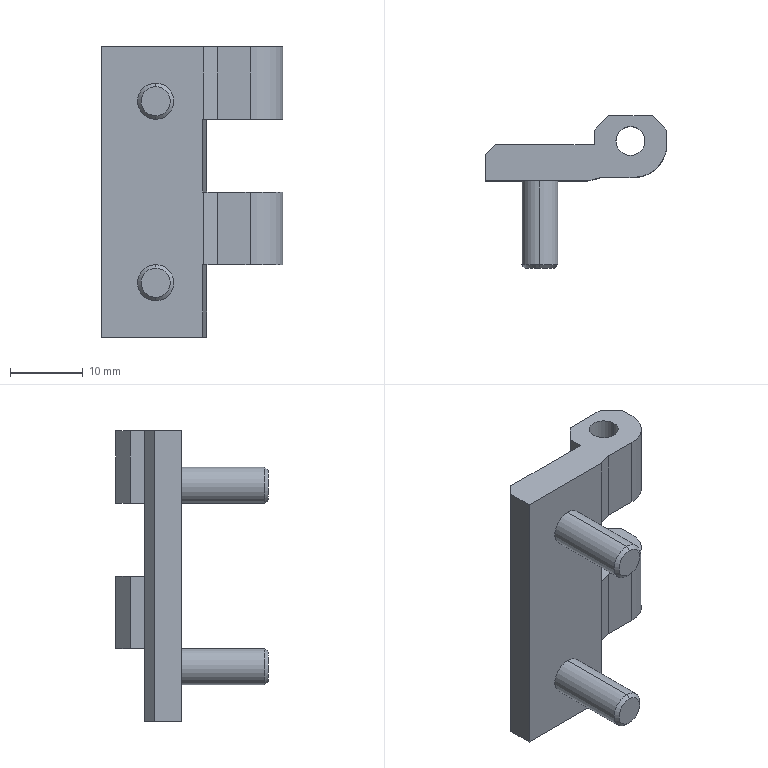Part | SolidWorks | features BaseBody 1 | 1 solid | 41 faces | box 25 x 21 x 40 mm | volume 4636 mm3 | plane 27 | cylinder 10 | cone 4 | commonest cylinder face diameters 4 x4 5 x4 9 x2
STEP:
#1=CARTESIAN_POINT('',(2.,5.5,20.));
#2=VERTEX_POINT('',#1);
#3=CARTESIAN_POINT('',(-2.,5.5,20.));
#4=VERTEX_POINT('',#3);
#5=CARTESIAN_POINT('',(0.,5.5,20.));
#6=DIRECTION('',(0.,0.,-1.));
#7=DIRECTION('',(-1.,0.,0.));
#8=AXIS2_PLACEMENT_3D('',#5,#6,#7);
#9=CIRCLE('',#8,2.);
#10=EDGE_CURVE('',#2,#4,#9,.T.);
#11=ORIENTED_EDGE('',*,*,#10,.F.);
#12=CARTESIAN_POINT('',(2.,5.5,10.));
#13=VERTEX_POINT('',#12);
#14=CARTESIAN_POINT('',(2.,5.5,20.));
#15=DIRECTION('',(0.,0.,-1.));
#16=VECTOR('',#15,1000.);
#17=LINE('',#14,#16);
#18=EDGE_CURVE('',#2,#13,#17,.T.);
#19=ORIENTED_EDGE('',*,*,#18,.T.);
#20=CARTESIAN_POINT('',(-2.,5.5,10.));
#21=VERTEX_POINT('',#20);
#22=CARTESIAN_POINT('',(0.,5.5,10.));
#23=DIRECTION('',(0.,0.,1.));
#24=DIRECTION('',(-1.,0.,0.));
#25=AXIS2_PLACEMENT_3D('',#22,#23,#24);
#26=CIRCLE('',#25,2.);
#27=EDGE_CURVE('',#21,#13,#26,.T.);
#28=ORIENTED_EDGE('',*,*,#27,.F.);
#29=CARTESIAN_POINT('',(-2.,5.5,20.));
#30=DIRECTION('',(0.,0.,-1.));
#31=VECTOR('',#30,1000.);
#32=LINE('',#29,#31);
#33=EDGE_CURVE('',#4,#21,#32,.T.);
#34=ORIENTED_EDGE('',*,*,#33,.F.);
#35=EDGE_LOOP('',(#11,#19,#28,#34));
#36=FACE_OUTER_BOUND('',#35,.T.);
#37=CARTESIAN_POINT('',(0.,5.5,20.));
#38=DIRECTION('',(0.,0.,-1.));
#39=DIRECTION('',(-1.,0.,0.));
#40=AXIS2_PLACEMENT_3D('',#37,#38,#39);
#41=CYLINDRICAL_SURFACE('',#40,2.);
#42=ADVANCED_FACE('',(#36),#41,.F.);
#43=CARTESIAN_POINT('',(-12.5,0.,10.));
#44=VERTEX_POINT('',#43);
#45=CARTESIAN_POINT('',(-12.5,0.,15.));
#46=VERTEX_POINT('',#45);
#47=CARTESIAN_POINT('',(-12.5,0.,12.5));
#48=DIRECTION('',(0.,-1.,0.));
#49=DIRECTION('',(0.,0.,-1.));
#50=AXIS2_PLACEMENT_3D('',#47,#48,#49);
#51=CIRCLE('',#50,2.5);
#52=EDGE_CURVE('',#44,#46,#51,.T.);
#53=ORIENTED_EDGE('',*,*,#52,.T.);
#54=CARTESIAN_POINT('',(-12.5,-11.509,15.));
#55=VERTEX_POINT('',#54);
#56=CARTESIAN_POINT('',(-12.5,-12.,15.));
#57=DIRECTION('',(0.,-1.,0.));
#58=VECTOR('',#57,1000.);
#59=LINE('',#56,#58);
#60=EDGE_CURVE('',#46,#55,#59,.T.);
#61=ORIENTED_EDGE('',*,*,#60,.T.);
#62=CARTESIAN_POINT('',(-12.5,-11.509,10.));
#63=VERTEX_POINT('',#62);
#64=CARTESIAN_POINT('',(-12.5,-11.509,12.5));
#65=DIRECTION('',(0.,1.,0.));
#66=DIRECTION('',(0.,0.,-1.));
#67=AXIS2_PLACEMENT_3D('',#64,#65,#66);
#68=CIRCLE('',#67,2.5);
#69=EDGE_CURVE('',#55,#63,#68,.T.);
#70=ORIENTED_EDGE('',*,*,#69,.T.);
#71=CARTESIAN_POINT('',(-12.5,-12.,10.));
#72=DIRECTION('',(0.,-1.,0.));
#73=VECTOR('',#72,1000.);
#74=LINE('',#71,#73);
#75=EDGE_CURVE('',#44,#63,#74,.T.);
#76=ORIENTED_EDGE('',*,*,#75,.F.);
#77=EDGE_LOOP('',(#53,#61,#70,#76));
#78=FACE_OUTER_BOUND('',#77,.T.);
#79=CARTESIAN_POINT('',(-12.5,-12.,12.5));
#80=DIRECTION('',(0.,-1.,0.));
#81=DIRECTION('',(0.,0.,-1.));
#82=AXIS2_PLACEMENT_3D('',#79,#80,#81);
#83=CYLINDRICAL_SURFACE('',#82,2.5);
#84=ADVANCED_FACE('',(#78),#83,.T.);
#85=CARTESIAN_POINT('',(-12.5,0.,-15.));
#86=VERTEX_POINT('',#85);
#87=CARTESIAN_POINT('',(-12.5,0.,-10.));
#88=VERTEX_POINT('',#87);
#89=CARTESIAN_POINT('',(-12.5,0.,-12.5));
#90=DIRECTION('',(0.,-1.,0.));
#91=DIRECTION('',(0.,0.,-1.));
#92=AXIS2_PLACEMENT_3D('',#89,#90,#91);
#93=CIRCLE('',#92,2.5);
#94=EDGE_CURVE('',#86,#88,#93,.T.);
#95=ORIENTED_EDGE('',*,*,#94,.T.);
#96=CARTESIAN_POINT('',(-12.5,-11.509,-10.));
#97=VERTEX_POINT('',#96);
#98=CARTESIAN_POINT('',(-12.5,-12.,-10.));
#99=DIRECTION('',(0.,-1.,0.));
#100=VECTOR('',#99,1000.);
#101=LINE('',#98,#100);
#102=EDGE_CURVE('',#88,#97,#101,.T.);
#103=ORIENTED_EDGE('',*,*,#102,.T.);
#104=CARTESIAN_POINT('',(-12.5,-11.509,-15.));
#105=VERTEX_POINT('',#104);
#106=CARTESIAN_POINT('',(-12.5,-11.509,-12.5));
#107=DIRECTION('',(0.,1.,0.));
#108=DIRECTION('',(0.,0.,-1.));
#109=AXIS2_PLACEMENT_3D('',#106,#107,#108);
#110=CIRCLE('',#109,2.5);
#111=EDGE_CURVE('',#97,#105,#110,.T.);
#112=ORIENTED_EDGE('',*,*,#111,.T.);
#113=CARTESIAN_POINT('',(-12.5,-12.,-15.));
#114=DIRECTION('',(0.,-1.,0.));
#115=VECTOR('',#114,1000.);
#116=LINE('',#113,#115);
#117=EDGE_CURVE('',#86,#105,#116,.T.);
#118=ORIENTED_EDGE('',*,*,#117,.F.);
#119=EDGE_LOOP('',(#95,#103,#112,#118));
#120=FACE_OUTER_BOUND('',#119,.T.);
#121=CARTESIAN_POINT('',(-12.5,-12.,-12.5));
#122=DIRECTION('',(0.,-1.,0.));
#123=DIRECTION('',(0.,0.,-1.));
#124=AXIS2_PLACEMENT_3D('',#121,#122,#123);
#125=CYLINDRICAL_SURFACE('',#124,2.5);
#126=ADVANCED_FACE('',(#120),#125,.T.);
#127=CARTESIAN_POINT('',(2.,5.5,-10.));
#128=VERTEX_POINT('',#127);
#129=CARTESIAN_POINT('',(-2.,5.5,-10.));
#130=VERTEX_POINT('',#129);
#131=CARTESIAN_POINT('',(0.,5.5,-10.));
#132=DIRECTION('',(0.,0.,-1.));
#133=DIRECTION('',(1.,0.,0.));
#134=AXIS2_PLACEMENT_3D('',#131,#132,#133);
#135=CIRCLE('',#134,2.);
#136=EDGE_CURVE('',#128,#130,#135,.T.);
#137=ORIENTED_EDGE('',*,*,#136,.T.);
#138=CARTESIAN_POINT('',(-2.,5.5,0.));
#139=VERTEX_POINT('',#138);
#140=CARTESIAN_POINT('',(-2.,5.5,-10.));
#141=DIRECTION('',(0.,0.,1.));
#142=VECTOR('',#141,1000.);
#143=LINE('',#140,#142);
#144=EDGE_CURVE('',#130,#139,#143,.T.);
#145=ORIENTED_EDGE('',*,*,#144,.T.);
#146=CARTESIAN_POINT('',(2.,5.5,0.));
#147=VERTEX_POINT('',#146);
#148=CARTESIAN_POINT('',(0.,5.5,0.));
#149=DIRECTION('',(0.,0.,-1.));
#150=DIRECTION('',(1.,0.,0.));
#151=AXIS2_PLACEMENT_3D('',#148,#149,#150);
#152=CIRCLE('',#151,2.);
#153=EDGE_CURVE('',#147,#139,#152,.T.);
#154=ORIENTED_EDGE('',*,*,#153,.F.);
#155=CARTESIAN_POINT('',(2.,5.5,-10.));
#156=DIRECTION('',(0.,0.,1.));
#157=VECTOR('',#156,1000.);
#158=LINE('',#155,#157);
#159=EDGE_CURVE('',#128,#147,#158,.T.);
#160=ORIENTED_EDGE('',*,*,#159,.F.);
#161=EDGE_LOOP('',(#137,#145,#154,#160));
#162=FACE_OUTER_BOUND('',#161,.T.);
#163=CARTESIAN_POINT('',(0.,5.5,-10.));
#164=DIRECTION('',(0.,0.,1.));
#165=DIRECTION('',(1.,0.,0.));
#166=AXIS2_PLACEMENT_3D('',#163,#164,#165);
#167=CYLINDRICAL_SURFACE('',#166,2.);
#168=ADVANCED_FACE('',(#162),#167,.F.);
#169=CARTESIAN_POINT('',(-12.5,-12.,14.509));
#170=VERTEX_POINT('',#169);
#171=CARTESIAN_POINT('',(-12.5,-12.,10.491));
#172=VERTEX_POINT('',#171);
#173=CARTESIAN_POINT('',(-12.5,-12.,12.5));
#174=DIRECTION('',(0.,1.,0.));
#175=DIRECTION('',(0.,0.,1.));
#176=AXIS2_PLACEMENT_3D('',#173,#174,#175);
#177=CIRCLE('',#176,2.009);
#178=EDGE_CURVE('',#170,#172,#177,.T.);
#179=ORIENTED_EDGE('',*,*,#178,.T.);
#180=CARTESIAN_POINT('',(-12.5,-11.51,10.));
#181=DIRECTION('',(0.,0.7071,-0.7071));
#182=VECTOR('',#181,1000.);
#183=LINE('',#180,#182);
#184=EDGE_CURVE('',#172,#63,#183,.T.);
#185=ORIENTED_EDGE('',*,*,#184,.T.);
#186=ORIENTED_EDGE('',*,*,#69,.F.);
#187=CARTESIAN_POINT('',(-12.5,-11.51,15.));
#188=DIRECTION('',(0.,0.7071,0.7071));
#189=VECTOR('',#188,1000.);
#190=LINE('',#187,#189);
#191=EDGE_CURVE('',#170,#55,#190,.T.);
#192=ORIENTED_EDGE('',*,*,#191,.F.);
#193=EDGE_LOOP('',(#179,#185,#186,#192));
#194=FACE_OUTER_BOUND('',#193,.T.);
#195=CARTESIAN_POINT('',(-12.5,-11.51,12.5));
#196=DIRECTION('',(0.,1.,0.));
#197=DIRECTION('',(0.,0.,1.));
#198=AXIS2_PLACEMENT_3D('',#195,#196,#197);
#199=CONICAL_SURFACE('',#198,2.5,0.7854);
#200=ADVANCED_FACE('',(#194),#199,.T.);
#201=CARTESIAN_POINT('',(-12.5,-12.,-10.49));
#202=VERTEX_POINT('',#201);
#203=CARTESIAN_POINT('',(-12.5,-12.,-14.51));
#204=VERTEX_POINT('',#203);
#205=CARTESIAN_POINT('',(-12.5,-12.,-12.5));
#206=DIRECTION('',(0.,1.,0.));
#207=DIRECTION('',(0.,0.,1.));
#208=AXIS2_PLACEMENT_3D('',#205,#206,#207);
#209=CIRCLE('',#208,2.01);
#210=EDGE_CURVE('',#202,#204,#209,.T.);
#211=ORIENTED_EDGE('',*,*,#210,.T.);
#212=CARTESIAN_POINT('',(-12.5,-11.509,-15.));
#213=DIRECTION('',(0.,0.7071,-0.7071));
#214=VECTOR('',#213,1000.);
#215=LINE('',#212,#214);
#216=EDGE_CURVE('',#204,#105,#215,.T.);
#217=ORIENTED_EDGE('',*,*,#216,.T.);
#218=ORIENTED_EDGE('',*,*,#111,.F.);
#219=CARTESIAN_POINT('',(-12.5,-11.509,-10.));
#220=DIRECTION('',(0.,0.7071,0.7071));
#221=VECTOR('',#220,1000.);
#222=LINE('',#219,#221);
#223=EDGE_CURVE('',#202,#97,#222,.T.);
#224=ORIENTED_EDGE('',*,*,#223,.F.);
#225=EDGE_LOOP('',(#211,#217,#218,#224));
#226=FACE_OUTER_BOUND('',#225,.T.);
#227=CARTESIAN_POINT('',(-12.5,-11.509,-12.5));
#228=DIRECTION('',(0.,1.,0.));
#229=DIRECTION('',(0.,0.,1.));
#230=AXIS2_PLACEMENT_3D('',#227,#228,#229);
#231=CONICAL_SURFACE('',#230,2.5,0.7854);
#232=ADVANCED_FACE('',(#226),#231,.T.);
#233=CARTESIAN_POINT('',(-5.,5.,20.));
#234=VERTEX_POINT('',#233);
#235=CARTESIAN_POINT('',(-18.6,5.,20.));
#236=VERTEX_POINT('',#235);
#237=CARTESIAN_POINT('',(-5.5,5.,20.));
#238=DIRECTION('',(-1.,0.,0.));
#239=VECTOR('',#238,1000.);
#240=LINE('',#237,#239);
#241=EDGE_CURVE('',#234,#236,#240,.T.);
#242=ORIENTED_EDGE('',*,*,#241,.F.);
#243=CARTESIAN_POINT('',(-5.,5.,10.));
#244=VERTEX_POINT('',#243);
#245=CARTESIAN_POINT('',(-5.,5.,20.));
#246=DIRECTION('',(0.,0.,1.));
#247=VECTOR('',#246,1000.);
#248=LINE('',#245,#247);
#249=EDGE_CURVE('',#244,#234,#248,.T.);
#250=ORIENTED_EDGE('',*,*,#249,.F.);
#251=CARTESIAN_POINT('',(-5.5,5.,10.));
#252=VERTEX_POINT('',#251);
#253=CARTESIAN_POINT('',(0.5,5.,10.));
#254=DIRECTION('',(-1.,0.,0.));
#255=VECTOR('',#254,1000.);
#256=LINE('',#253,#255);
#257=EDGE_CURVE('',#244,#252,#256,.T.);
#258=ORIENTED_EDGE('',*,*,#257,.T.);
#259=CARTESIAN_POINT('',(-5.5,5.,0.));
#260=VERTEX_POINT('',#259);
#261=CARTESIAN_POINT('',(-5.5,5.,20.));
#262=DIRECTION('',(0.,0.,1.));
#263=VECTOR('',#262,1000.);
#264=LINE('',#261,#263);
#265=EDGE_CURVE('',#260,#252,#264,.T.);
#266=ORIENTED_EDGE('',*,*,#265,.F.);
#267=CARTESIAN_POINT('',(-5.,5.,0.));
#268=VERTEX_POINT('',#267);
#269=CARTESIAN_POINT('',(0.5,5.,0.));
#270=DIRECTION('',(-1.,0.,0.));
#271=VECTOR('',#270,1000.);
#272=LINE('',#269,#271);
#273=EDGE_CURVE('',#268,#260,#272,.T.);
#274=ORIENTED_EDGE('',*,*,#273,.F.);
#275=CARTESIAN_POINT('',(-5.,5.,-10.));
#276=VERTEX_POINT('',#275);
#277=CARTESIAN_POINT('',(-5.,5.,20.));
#278=DIRECTION('',(0.,0.,1.));
#279=VECTOR('',#278,1000.);
#280=LINE('',#277,#279);
#281=EDGE_CURVE('',#276,#268,#280,.T.);
#282=ORIENTED_EDGE('',*,*,#281,.F.);
#283=CARTESIAN_POINT('',(-5.5,5.,-10.));
#284=VERTEX_POINT('',#283);
#285=CARTESIAN_POINT('',(0.5,5.,-10.));
#286=DIRECTION('',(-1.,0.,0.));
#287=VECTOR('',#286,1000.);
#288=LINE('',#285,#287);
#289=EDGE_CURVE('',#276,#284,#288,.T.);
#290=ORIENTED_EDGE('',*,*,#289,.T.);
#291=CARTESIAN_POINT('',(-5.5,5.,-20.));
#292=VERTEX_POINT('',#291);
#293=CARTESIAN_POINT('',(-5.5,5.,20.));
#294=DIRECTION('',(0.,0.,1.));
#295=VECTOR('',#294,1000.);
#296=LINE('',#293,#295);
#297=EDGE_CURVE('',#292,#284,#296,.T.);
#298=ORIENTED_EDGE('',*,*,#297,.F.);
#299=CARTESIAN_POINT('',(-18.6,5.,-20.));
#300=VERTEX_POINT('',#299);
#301=CARTESIAN_POINT('',(-5.5,5.,-20.));
#302=DIRECTION('',(1.,0.,0.));
#303=VECTOR('',#302,1000.);
#304=LINE('',#301,#303);
#305=EDGE_CURVE('',#300,#292,#304,.T.);
#306=ORIENTED_EDGE('',*,*,#305,.F.);
#307=CARTESIAN_POINT('',(-18.6,5.,20.));
#308=DIRECTION('',(0.,0.,-1.));
#309=VECTOR('',#308,1000.);
#310=LINE('',#307,#309);
#311=EDGE_CURVE('',#236,#300,#310,.T.);
#312=ORIENTED_EDGE('',*,*,#311,.F.);
#313=EDGE_LOOP('',(#242,#250,#258,#266,#274,#282,#290,#298,#306,#312));
#314=FACE_OUTER_BOUND('',#313,.T.);
#315=CARTESIAN_POINT('',(-5.5,5.,20.));
#316=DIRECTION('',(0.,-1.,0.));
#317=DIRECTION('',(0.,0.,-1.));
#318=AXIS2_PLACEMENT_3D('',#315,#316,#317);
#319=PLANE('',#318);
#320=ADVANCED_FACE('',(#314),#319,.F.);
#321=CARTESIAN_POINT('',(-20.,3.6,20.));
#322=VERTEX_POINT('',#321);
#323=CARTESIAN_POINT('',(-20.,3.6,-20.));
#324=VERTEX_POINT('',#323);
#325=CARTESIAN_POINT('',(-20.,3.6,20.));
#326=DIRECTION('',(0.,0.,-1.));
#327=VECTOR('',#326,1000.);
#328=LINE('',#325,#327);
#329=EDGE_CURVE('',#322,#324,#328,.T.);
#330=ORIENTED_EDGE('',*,*,#329,.F.);
#331=CARTESIAN_POINT('',(-18.6,5.,20.));
#332=DIRECTION('',(-0.7071,-0.7071,0.));
#333=VECTOR('',#332,1000.);
#334=LINE('',#331,#333);
#335=EDGE_CURVE('',#236,#322,#334,.T.);
#336=ORIENTED_EDGE('',*,*,#335,.F.);
#337=ORIENTED_EDGE('',*,*,#311,.T.);
#338=CARTESIAN_POINT('',(-18.6,5.,-20.));
#339=DIRECTION('',(0.7071,0.7071,0.));
#340=VECTOR('',#339,1000.);
#341=LINE('',#338,#340);
#342=EDGE_CURVE('',#324,#300,#341,.T.);
#343=ORIENTED_EDGE('',*,*,#342,.F.);
#344=EDGE_LOOP('',(#330,#336,#337,#343));
#345=FACE_OUTER_BOUND('',#344,.T.);
#346=CARTESIAN_POINT('',(-18.6,5.,20.));
#347=DIRECTION('',(0.7071,-0.7071,0.));
#348=DIRECTION('',(0.7071,0.7071,0.));
#349=AXIS2_PLACEMENT_3D('',#346,#347,#348);
#350=PLANE('',#349);
#351=ADVANCED_FACE('',(#345),#350,.F.);
#352=CARTESIAN_POINT('',(0.,5.5,20.));
#353=DIRECTION('',(0.,0.,-1.));
#354=DIRECTION('',(-1.,0.,0.));
#355=AXIS2_PLACEMENT_3D('',#352,#353,#354);
#356=CIRCLE('',#355,2.);
#357=EDGE_CURVE('',#4,#2,#356,.T.);
#358=ORIENTED_EDGE('',*,*,#357,.T.);
#359=ORIENTED_EDGE('',*,*,#10,.T.);
#360=EDGE_LOOP('',(#358,#359));
#361=FACE_BOUND('',#360,.T.);
#362=CARTESIAN_POINT('',(-3.,9.,20.));
#363=VERTEX_POINT('',#362);
#364=CARTESIAN_POINT('',(-5.,7.,20.));
#365=VERTEX_POINT('',#364);
#366=CARTESIAN_POINT('',(-3.,9.,20.));
#367=DIRECTION('',(-0.7071,-0.7071,0.));
#368=VECTOR('',#367,1000.);
#369=LINE('',#366,#368);
#370=EDGE_CURVE('',#363,#365,#369,.T.);
#371=ORIENTED_EDGE('',*,*,#370,.T.);
#372=CARTESIAN_POINT('',(-5.,0.,20.));
#373=DIRECTION('',(0.,-1.,0.));
#374=VECTOR('',#373,1000.);
#375=LINE('',#372,#374);
#376=EDGE_CURVE('',#365,#234,#375,.T.);
#377=ORIENTED_EDGE('',*,*,#376,.T.);
#378=ORIENTED_EDGE('',*,*,#241,.T.);
#379=ORIENTED_EDGE('',*,*,#335,.T.);
#380=CARTESIAN_POINT('',(-20.,0.,20.));
#381=VERTEX_POINT('',#380);
#382=CARTESIAN_POINT('',(-20.,0.,20.));
#383=DIRECTION('',(0.,-1.,0.));
#384=VECTOR('',#383,1000.);
#385=LINE('',#382,#384);
#386=EDGE_CURVE('',#322,#381,#385,.T.);
#387=ORIENTED_EDGE('',*,*,#386,.T.);
#388=CARTESIAN_POINT('',(-5.866,0.,20.));
#389=VERTEX_POINT('',#388);
#390=CARTESIAN_POINT('',(0.,0.,20.));
#391=DIRECTION('',(1.,0.,0.));
#392=VECTOR('',#391,1000.);
#393=LINE('',#390,#392);
#394=EDGE_CURVE('',#381,#389,#393,.T.);
#395=ORIENTED_EDGE('',*,*,#394,.T.);
#396=CARTESIAN_POINT('',(-4.,0.5,20.));
#397=VERTEX_POINT('',#396);
#398=CARTESIAN_POINT('',(-5.866,0.,20.));
#399=DIRECTION('',(0.9659,0.2588,0.));
#400=VECTOR('',#399,1000.);
#401=LINE('',#398,#400);
#402=EDGE_CURVE('',#389,#397,#401,.T.);
#403=ORIENTED_EDGE('',*,*,#402,.T.);
#404=CARTESIAN_POINT('',(0.5,0.5,20.));
#405=VERTEX_POINT('',#404);
#406=CARTESIAN_POINT('',(0.,0.5,20.));
#407=DIRECTION('',(1.,0.,0.));
#408=VECTOR('',#407,1000.);
#409=LINE('',#406,#408);
#410=EDGE_CURVE('',#397,#405,#409,.T.);
#411=ORIENTED_EDGE('',*,*,#410,.T.);
#412=CARTESIAN_POINT('',(5.,5.,20.));
#413=VERTEX_POINT('',#412);
#414=CARTESIAN_POINT('',(0.5,5.,20.));
#415=DIRECTION('',(0.,0.,1.));
#416=DIRECTION('',(-1.,0.,0.));
#417=AXIS2_PLACEMENT_3D('',#414,#415,#416);
#418=CIRCLE('',#417,4.5);
#419=EDGE_CURVE('',#405,#413,#418,.T.);
#420=ORIENTED_EDGE('',*,*,#419,.T.);
#421=CARTESIAN_POINT('',(5.,7.,20.));
#422=VERTEX_POINT('',#421);
#423=CARTESIAN_POINT('',(5.,0.,20.));
#424=DIRECTION('',(0.,1.,0.));
#425=VECTOR('',#424,1000.);
#426=LINE('',#423,#425);
#427=EDGE_CURVE('',#413,#422,#426,.T.);
#428=ORIENTED_EDGE('',*,*,#427,.T.);
#429=CARTESIAN_POINT('',(3.,9.,20.));
#430=VERTEX_POINT('',#429);
#431=CARTESIAN_POINT('',(5.,7.,20.));
#432=DIRECTION('',(-0.7071,0.7071,0.));
#433=VECTOR('',#432,1000.);
#434=LINE('',#431,#433);
#435=EDGE_CURVE('',#422,#430,#434,.T.);
#436=ORIENTED_EDGE('',*,*,#435,.T.);
#437=CARTESIAN_POINT('',(0.,9.,20.));
#438=DIRECTION('',(-1.,0.,0.));
#439=VECTOR('',#438,1000.);
#440=LINE('',#437,#439);
#441=EDGE_CURVE('',#430,#363,#440,.T.);
#442=ORIENTED_EDGE('',*,*,#441,.T.);
#443=EDGE_LOOP('',(#371,#377,#378,#379,#387,#395,#403,#411,#420,#428,#436,#442));
#444=FACE_OUTER_BOUND('',#443,.T.);
#445=CARTESIAN_POINT('',(0.,0.,20.));
#446=DIRECTION('',(0.,0.,1.));
#447=DIRECTION('',(1.,0.,0.));
#448=AXIS2_PLACEMENT_3D('',#445,#446,#447);
#449=PLANE('',#448);
#450=ADVANCED_FACE('',(#361,#444),#449,.T.);
#451=ORIENTED_EDGE('',*,*,#249,.T.);
#452=ORIENTED_EDGE('',*,*,#376,.F.);
#453=CARTESIAN_POINT('',(-5.,7.,10.));
#454=VERTEX_POINT('',#453);
#455=CARTESIAN_POINT('',(-5.,7.,20.));
#456=DIRECTION('',(0.,0.,1.));
#457=VECTOR('',#456,1000.);
#458=LINE('',#455,#457);
#459=EDGE_CURVE('',#454,#365,#458,.T.);
#460=ORIENTED_EDGE('',*,*,#459,.F.);
#461=CARTESIAN_POINT('',(-5.,7.,10.));
#462=DIRECTION('',(0.,1.,0.));
#463=VECTOR('',#462,1000.);
#464=LINE('',#461,#463);
#465=EDGE_CURVE('',#244,#454,#464,.T.);
#466=ORIENTED_EDGE('',*,*,#465,.F.);
#467=EDGE_LOOP('',(#451,#452,#460,#466));
#468=FACE_OUTER_BOUND('',#467,.T.);
#469=CARTESIAN_POINT('',(-5.,7.,20.));
#470=DIRECTION('',(1.,0.,0.));
#471=DIRECTION('',(0.,0.,-1.));
#472=AXIS2_PLACEMENT_3D('',#469,#470,#471);
#473=PLANE('',#472);
#474=ADVANCED_FACE('',(#468),#473,.F.);
#475=CARTESIAN_POINT('',(-6.,0.,0.));
#476=VERTEX_POINT('',#475);
#477=CARTESIAN_POINT('',(-6.,0.,10.));
#478=VERTEX_POINT('',#477);
#479=CARTESIAN_POINT('',(-6.,0.,20.));
#480=DIRECTION('',(0.,0.,1.));
#481=VECTOR('',#480,1000.);
#482=LINE('',#479,#481);
#483=EDGE_CURVE('',#476,#478,#482,.T.);
#484=ORIENTED_EDGE('',*,*,#483,.F.);
#485=CARTESIAN_POINT('',(-6.,0.,0.));
#486=DIRECTION('',(-0.0995,-0.995,0.));
#487=VECTOR('',#486,1000.);
#488=LINE('',#485,#487);
#489=EDGE_CURVE('',#260,#476,#488,.T.);
#490=ORIENTED_EDGE('',*,*,#489,.F.);
#491=ORIENTED_EDGE('',*,*,#265,.T.);
#492=CARTESIAN_POINT('',(-6.,0.,10.));
#493=DIRECTION('',(0.0995,0.995,0.));
#494=VECTOR('',#493,1000.);
#495=LINE('',#492,#494);
#496=EDGE_CURVE('',#478,#252,#495,.T.);
#497=ORIENTED_EDGE('',*,*,#496,.F.);
#498=EDGE_LOOP('',(#484,#490,#491,#497));
#499=FACE_OUTER_BOUND('',#498,.T.);
#500=CARTESIAN_POINT('',(-6.,0.,20.));
#501=DIRECTION('',(-0.995,0.0995,0.));
#502=DIRECTION('',(-0.0995,-0.995,0.));
#503=AXIS2_PLACEMENT_3D('',#500,#501,#502);
#504=PLANE('',#503);
#505=ADVANCED_FACE('',(#499),#504,.F.);
#506=CARTESIAN_POINT('',(-5.,7.,-10.));
#507=VERTEX_POINT('',#506);
#508=CARTESIAN_POINT('',(-5.,7.,-10.));
#509=DIRECTION('',(0.,-1.,0.));
#510=VECTOR('',#509,1000.);
#511=LINE('',#508,#510);
#512=EDGE_CURVE('',#507,#276,#511,.T.);
#513=ORIENTED_EDGE('',*,*,#512,.T.);
#514=ORIENTED_EDGE('',*,*,#281,.T.);
#515=CARTESIAN_POINT('',(-5.,7.,0.));
#516=VERTEX_POINT('',#515);
#517=CARTESIAN_POINT('',(-5.,7.,0.));
#518=DIRECTION('',(0.,1.,0.));
#519=VECTOR('',#518,1000.);
#520=LINE('',#517,#519);
#521=EDGE_CURVE('',#268,#516,#520,.T.);
#522=ORIENTED_EDGE('',*,*,#521,.T.);
#523=CARTESIAN_POINT('',(-5.,7.,-10.));
#524=DIRECTION('',(0.,0.,-1.));
#525=VECTOR('',#524,1000.);
#526=LINE('',#523,#525);
#527=EDGE_CURVE('',#516,#507,#526,.T.);
#528=ORIENTED_EDGE('',*,*,#527,.T.);
#529=EDGE_LOOP('',(#513,#514,#522,#528));
#530=FACE_OUTER_BOUND('',#529,.T.);
#531=CARTESIAN_POINT('',(-5.,7.,-10.));
#532=DIRECTION('',(-1.,0.,0.));
#533=DIRECTION('',(0.,0.,1.));
#534=AXIS2_PLACEMENT_3D('',#531,#532,#533);
#535=PLANE('',#534);
#536=ADVANCED_FACE('',(#530),#535,.T.);
#537=CARTESIAN_POINT('',(-6.,0.,-20.));
#538=VERTEX_POINT('',#537);
#539=CARTESIAN_POINT('',(-6.,0.,-10.));
#540=VERTEX_POINT('',#539);
#541=CARTESIAN_POINT('',(-6.,0.,20.));
#542=DIRECTION('',(0.,0.,1.));
#543=VECTOR('',#542,1000.);
#544=LINE('',#541,#543);
#545=EDGE_CURVE('',#538,#540,#544,.T.);
#546=ORIENTED_EDGE('',*,*,#545,.F.);
#547=CARTESIAN_POINT('',(-6.,0.,-20.));
#548=DIRECTION('',(-0.0995,-0.995,0.));
#549=VECTOR('',#548,1000.);
#550=LINE('',#547,#549);
#551=EDGE_CURVE('',#292,#538,#550,.T.);
#552=ORIENTED_EDGE('',*,*,#551,.F.);
#553=ORIENTED_EDGE('',*,*,#297,.T.);
#554=CARTESIAN_POINT('',(-6.,0.,-10.));
#555=DIRECTION('',(0.0995,0.995,0.));
#556=VECTOR('',#555,1000.);
#557=LINE('',#554,#556);
#558=EDGE_CURVE('',#540,#284,#557,.T.);
#559=ORIENTED_EDGE('',*,*,#558,.F.);
#560=EDGE_LOOP('',(#546,#552,#553,#559));
#561=FACE_OUTER_BOUND('',#560,.T.);
#562=CARTESIAN_POINT('',(-6.,0.,20.));
#563=DIRECTION('',(-0.995,0.0995,0.));
#564=DIRECTION('',(-0.0995,-0.995,0.));
#565=AXIS2_PLACEMENT_3D('',#562,#563,#564);
#566=PLANE('',#565);
#567=ADVANCED_FACE('',(#561),#566,.F.);
#568=ORIENTED_EDGE('',*,*,#305,.T.);
#569=ORIENTED_EDGE('',*,*,#551,.T.);
#570=CARTESIAN_POINT('',(-20.,0.,-20.));
#571=VERTEX_POINT('',#570);
#572=CARTESIAN_POINT('',(0.,0.,-20.));
#573=DIRECTION('',(1.,0.,0.));
#574=VECTOR('',#573,1000.);
#575=LINE('',#572,#574);
#576=EDGE_CURVE('',#571,#538,#575,.T.);
#577=ORIENTED_EDGE('',*,*,#576,.F.);
#578=CARTESIAN_POINT('',(-20.,0.,-20.));
#579=DIRECTION('',(0.,-1.,0.));
#580=VECTOR('',#579,1000.);
#581=LINE('',#578,#580);
#582=EDGE_CURVE('',#324,#571,#581,.T.);
#583=ORIENTED_EDGE('',*,*,#582,.F.);
#584=ORIENTED_EDGE('',*,*,#342,.T.);
#585=EDGE_LOOP('',(#568,#569,#577,#583,#584));
#586=FACE_OUTER_BOUND('',#585,.T.);
#587=CARTESIAN_POINT('',(0.,0.,-20.));
#588=DIRECTION('',(0.,0.,1.));
#589=DIRECTION('',(1.,0.,0.));
#590=AXIS2_PLACEMENT_3D('',#587,#588,#589);
#591=PLANE('',#590);
#592=ADVANCED_FACE('',(#586),#591,.F.);
#593=CARTESIAN_POINT('',(-20.,0.,20.));
#594=DIRECTION('',(0.,0.,-1.));
#595=VECTOR('',#594,1000.);
#596=LINE('',#593,#595);
#597=EDGE_CURVE('',#381,#571,#596,.T.);
#598=ORIENTED_EDGE('',*,*,#597,.F.);
#599=ORIENTED_EDGE('',*,*,#386,.F.);
#600=ORIENTED_EDGE('',*,*,#329,.T.);
#601=ORIENTED_EDGE('',*,*,#582,.T.);
#602=EDGE_LOOP('',(#598,#599,#600,#601));
#603=FACE_OUTER_BOUND('',#602,.T.);
#604=CARTESIAN_POINT('',(-20.,3.6,20.));
#605=DIRECTION('',(1.,0.,0.));
#606=DIRECTION('',(0.,0.,-1.));
#607=AXIS2_PLACEMENT_3D('',#604,#605,#606);
#608=PLANE('',#607);
#609=ADVANCED_FACE('',(#603),#608,.F.);
#610=ORIENTED_EDGE('',*,*,#18,.F.);
#611=ORIENTED_EDGE('',*,*,#357,.F.);
#612=ORIENTED_EDGE('',*,*,#33,.T.);
#613=CARTESIAN_POINT('',(0.,5.5,10.));
#614=DIRECTION('',(0.,0.,1.));
#615=DIRECTION('',(-1.,0.,0.));
#616=AXIS2_PLACEMENT_3D('',#613,#614,#615);
#617=CIRCLE('',#616,2.);
#618=EDGE_CURVE('',#13,#21,#617,.T.);
#619=ORIENTED_EDGE('',*,*,#618,.F.);
#620=EDGE_LOOP('',(#610,#611,#612,#619));
#621=FACE_OUTER_BOUND('',#620,.T.);
#622=CARTESIAN_POINT('',(0.,5.5,20.));
#623=DIRECTION('',(0.,0.,-1.));
#624=DIRECTION('',(-1.,0.,0.));
#625=AXIS2_PLACEMENT_3D('',#622,#623,#624);
#626=CYLINDRICAL_SURFACE('',#625,2.);
#627=ADVANCED_FACE('',(#621),#626,.F.);
#628=ORIENTED_EDGE('',*,*,#459,.T.);
#629=ORIENTED_EDGE('',*,*,#370,.F.);
#630=CARTESIAN_POINT('',(-3.,9.,10.));
#631=VERTEX_POINT('',#630);
#632=CARTESIAN_POINT('',(-3.,9.,20.));
#633=DIRECTION('',(0.,0.,1.));
#634=VECTOR('',#633,1000.);
#635=LINE('',#632,#634);
#636=EDGE_CURVE('',#631,#363,#635,.T.);
#637=ORIENTED_EDGE('',*,*,#636,.F.);
#638=CARTESIAN_POINT('',(-3.,9.,10.));
#639=DIRECTION('',(0.7071,0.7071,0.));
#640=VECTOR('',#639,1000.);
#641=LINE('',#638,#640);
#642=EDGE_CURVE('',#454,#631,#641,.T.);
#643=ORIENTED_EDGE('',*,*,#642,.F.);
#644=EDGE_LOOP('',(#628,#629,#637,#643));
#645=FACE_OUTER_BOUND('',#644,.T.);
#646=CARTESIAN_POINT('',(-3.,9.,20.));
#647=DIRECTION('',(0.7071,-0.7071,0.));
#648=DIRECTION('',(0.7071,0.7071,0.));
#649=AXIS2_PLACEMENT_3D('',#646,#647,#648);
#650=PLANE('',#649);
#651=ADVANCED_FACE('',(#645),#650,.F.);
#652=ORIENTED_EDGE('',*,*,#636,.T.);
#653=ORIENTED_EDGE('',*,*,#441,.F.);
#654=CARTESIAN_POINT('',(3.,9.,10.));
#655=VERTEX_POINT('',#654);
#656=CARTESIAN_POINT('',(3.,9.,20.));
#657=DIRECTION('',(0.,0.,1.));
#658=VECTOR('',#657,1000.);
#659=LINE('',#656,#658);
#660=EDGE_CURVE('',#655,#430,#659,.T.);
#661=ORIENTED_EDGE('',*,*,#660,.F.);
#662=CARTESIAN_POINT('',(3.,9.,10.));
#663=DIRECTION('',(1.,0.,0.));
#664=VECTOR('',#663,1000.);
#665=LINE('',#662,#664);
#666=EDGE_CURVE('',#631,#655,#665,.T.);
#667=ORIENTED_EDGE('',*,*,#666,.F.);
#668=EDGE_LOOP('',(#652,#653,#661,#667));
#669=FACE_OUTER_BOUND('',#668,.T.);
#670=CARTESIAN_POINT('',(3.,9.,20.));
#671=DIRECTION('',(0.,-1.,0.));
#672=DIRECTION('',(0.,0.,-1.));
#673=AXIS2_PLACEMENT_3D('',#670,#671,#672);
#674=PLANE('',#673);
#675=ADVANCED_FACE('',(#669),#674,.F.);
#676=ORIENTED_EDGE('',*,*,#660,.T.);
#677=ORIENTED_EDGE('',*,*,#435,.F.);
#678=CARTESIAN_POINT('',(5.,7.,10.));
#679=VERTEX_POINT('',#678);
#680=CARTESIAN_POINT('',(5.,7.,20.));
#681=DIRECTION('',(0.,0.,1.));
#682=VECTOR('',#681,1000.);
#683=LINE('',#680,#682);
#684=EDGE_CURVE('',#679,#422,#683,.T.);
#685=ORIENTED_EDGE('',*,*,#684,.F.);
#686=CARTESIAN_POINT('',(5.,7.,10.));
#687=DIRECTION('',(0.7071,-0.7071,0.));
#688=VECTOR('',#687,1000.);
#689=LINE('',#686,#688);
#690=EDGE_CURVE('',#655,#679,#689,.T.);
#691=ORIENTED_EDGE('',*,*,#690,.F.);
#692=EDGE_LOOP('',(#676,#677,#685,#691));
#693=FACE_OUTER_BOUND('',#692,.T.);
#694=CARTESIAN_POINT('',(5.,7.,20.));
#695=DIRECTION('',(-0.7071,-0.7071,0.));
#696=DIRECTION('',(0.7071,-0.7071,0.));
#697=AXIS2_PLACEMENT_3D('',#694,#695,#696);
#698=PLANE('',#697);
#699=ADVANCED_FACE('',(#693),#698,.F.);
#700=ORIENTED_EDGE('',*,*,#684,.T.);
#701=ORIENTED_EDGE('',*,*,#427,.F.);
#702=CARTESIAN_POINT('',(5.,5.,10.));
#703=VERTEX_POINT('',#702);
#704=CARTESIAN_POINT('',(5.,5.,20.));
#705=DIRECTION('',(0.,0.,1.));
#706=VECTOR('',#705,1000.);
#707=LINE('',#704,#706);
#708=EDGE_CURVE('',#703,#413,#707,.T.);
#709=ORIENTED_EDGE('',*,*,#708,.F.);
#710=CARTESIAN_POINT('',(5.,5.,10.));
#711=DIRECTION('',(0.,-1.,0.));
#712=VECTOR('',#711,1000.);
#713=LINE('',#710,#712);
#714=EDGE_CURVE('',#679,#703,#713,.T.);
#715=ORIENTED_EDGE('',*,*,#714,.F.);
#716=EDGE_LOOP('',(#700,#701,#709,#715));
#717=FACE_OUTER_BOUND('',#716,.T.);
#718=CARTESIAN_POINT('',(5.,5.,20.));
#719=DIRECTION('',(-1.,0.,0.));
#720=DIRECTION('',(0.,0.,1.));
#721=AXIS2_PLACEMENT_3D('',#718,#719,#720);
#722=PLANE('',#721);
#723=ADVANCED_FACE('',(#717),#722,.F.);
#724=ORIENTED_EDGE('',*,*,#419,.F.);
#725=CARTESIAN_POINT('',(0.5,0.5,10.));
#726=VERTEX_POINT('',#725);
#727=CARTESIAN_POINT('',(0.5,0.5,20.));
#728=DIRECTION('',(0.,0.,-1.));
#729=VECTOR('',#728,1000.);
#730=LINE('',#727,#729);
#731=EDGE_CURVE('',#405,#726,#730,.T.);
#732=ORIENTED_EDGE('',*,*,#731,.T.);
#733=CARTESIAN_POINT('',(0.5,5.,10.));
#734=DIRECTION('',(0.,0.,1.));
#735=DIRECTION('',(-1.,0.,0.));
#736=AXIS2_PLACEMENT_3D('',#733,#734,#735);
#737=CIRCLE('',#736,4.5);
#738=EDGE_CURVE('',#726,#703,#737,.T.);
#739=ORIENTED_EDGE('',*,*,#738,.T.);
#740=ORIENTED_EDGE('',*,*,#708,.T.);
#741=EDGE_LOOP('',(#724,#732,#739,#740));
#742=FACE_OUTER_BOUND('',#741,.T.);
#743=CARTESIAN_POINT('',(0.5,5.,20.));
#744=DIRECTION('',(0.,0.,-1.));
#745=DIRECTION('',(-1.,0.,0.));
#746=AXIS2_PLACEMENT_3D('',#743,#744,#745);
#747=CYLINDRICAL_SURFACE('',#746,4.5);
#748=ADVANCED_FACE('',(#742),#747,.T.);
#749=ORIENTED_EDGE('',*,*,#731,.F.);
#750=ORIENTED_EDGE('',*,*,#410,.F.);
#751=CARTESIAN_POINT('',(-4.,0.5,10.));
#752=VERTEX_POINT('',#751);
#753=CARTESIAN_POINT('',(-4.,0.5,20.));
#754=DIRECTION('',(0.,0.,1.));
#755=VECTOR('',#754,1000.);
#756=LINE('',#753,#755);
#757=EDGE_CURVE('',#752,#397,#756,.T.);
#758=ORIENTED_EDGE('',*,*,#757,.F.);
#759=CARTESIAN_POINT('',(-4.,0.5,10.));
#760=DIRECTION('',(-1.,0.,0.));
#761=VECTOR('',#760,1000.);
#762=LINE('',#759,#761);
#763=EDGE_CURVE('',#726,#752,#762,.T.);
#764=ORIENTED_EDGE('',*,*,#763,.F.);
#765=EDGE_LOOP('',(#749,#750,#758,#764));
#766=FACE_OUTER_BOUND('',#765,.T.);
#767=CARTESIAN_POINT('',(-4.,0.5,20.));
#768=DIRECTION('',(0.,1.,0.));
#769=DIRECTION('',(0.,0.,1.));
#770=AXIS2_PLACEMENT_3D('',#767,#768,#769);
#771=PLANE('',#770);
#772=ADVANCED_FACE('',(#766),#771,.F.);
#773=ORIENTED_EDGE('',*,*,#757,.T.);
#774=ORIENTED_EDGE('',*,*,#402,.F.);
#775=CARTESIAN_POINT('',(-5.866,0.,10.));
#776=VERTEX_POINT('',#775);
#777=CARTESIAN_POINT('',(-5.866,0.,20.));
#778=DIRECTION('',(0.,0.,1.));
#779=VECTOR('',#778,1000.);
#780=LINE('',#777,#779);
#781=EDGE_CURVE('',#776,#389,#780,.T.);
#782=ORIENTED_EDGE('',*,*,#781,.F.);
#783=CARTESIAN_POINT('',(-5.866,0.,10.));
#784=DIRECTION('',(-0.9659,-0.2588,0.));
#785=VECTOR('',#784,1000.);
#786=LINE('',#783,#785);
#787=EDGE_CURVE('',#752,#776,#786,.T.);
#788=ORIENTED_EDGE('',*,*,#787,.F.);
#789=EDGE_LOOP('',(#773,#774,#782,#788));
#790=FACE_OUTER_BOUND('',#789,.T.);
#791=CARTESIAN_POINT('',(-5.866,0.,20.));
#792=DIRECTION('',(-0.2588,0.9659,0.));
#793=DIRECTION('',(-0.9659,-0.2588,0.));
#794=AXIS2_PLACEMENT_3D('',#791,#792,#793);
#795=PLANE('',#794);
#796=ADVANCED_FACE('',(#790),#795,.F.);
#797=ORIENTED_EDGE('',*,*,#394,.F.);
#798=ORIENTED_EDGE('',*,*,#597,.T.);
#799=ORIENTED_EDGE('',*,*,#576,.T.);
#800=ORIENTED_EDGE('',*,*,#545,.T.);
#801=CARTESIAN_POINT('',(-5.866,0.,-10.));
#802=VERTEX_POINT('',#801);
#803=CARTESIAN_POINT('',(-20.,0.,-10.));
#804=DIRECTION('',(-1.,0.,0.));
#805=VECTOR('',#804,1000.);
#806=LINE('',#803,#805);
#807=EDGE_CURVE('',#802,#540,#806,.T.);
#808=ORIENTED_EDGE('',*,*,#807,.F.);
#809=CARTESIAN_POINT('',(-5.866,0.,0.));
#810=VERTEX_POINT('',#809);
#811=CARTESIAN_POINT('',(-5.866,0.,20.));
#812=DIRECTION('',(0.,0.,-1.));
#813=VECTOR('',#812,1000.);
#814=LINE('',#811,#813);
#815=EDGE_CURVE('',#810,#802,#814,.T.);
#816=ORIENTED_EDGE('',*,*,#815,.F.);
#817=CARTESIAN_POINT('',(-20.,0.,0.));
#818=DIRECTION('',(1.,0.,0.));
#819=VECTOR('',#818,1000.);
#820=LINE('',#817,#819);
#821=EDGE_CURVE('',#476,#810,#820,.T.);
#822=ORIENTED_EDGE('',*,*,#821,.F.);
#823=ORIENTED_EDGE('',*,*,#483,.T.);
#824=CARTESIAN_POINT('',(-20.,0.,10.));
#825=DIRECTION('',(-1.,0.,0.));
#826=VECTOR('',#825,1000.);
#827=LINE('',#824,#826);
#828=EDGE_CURVE('',#776,#478,#827,.T.);
#829=ORIENTED_EDGE('',*,*,#828,.F.);
#830=ORIENTED_EDGE('',*,*,#781,.T.);
#831=EDGE_LOOP('',(#797,#798,#799,#800,#808,#816,#822,#823,#829,#830));
#832=FACE_OUTER_BOUND('',#831,.T.);
#833=ORIENTED_EDGE('',*,*,#52,.F.);
#834=CARTESIAN_POINT('',(-12.5,0.,12.5));
#835=DIRECTION('',(0.,-1.,0.));
#836=DIRECTION('',(0.,0.,-1.));
#837=AXIS2_PLACEMENT_3D('',#834,#835,#836);
#838=CIRCLE('',#837,2.5);
#839=EDGE_CURVE('',#46,#44,#838,.T.);
#840=ORIENTED_EDGE('',*,*,#839,.F.);
#841=EDGE_LOOP('',(#833,#840));
#842=FACE_BOUND('',#841,.T.);
#843=ORIENTED_EDGE('',*,*,#94,.F.);
#844=CARTESIAN_POINT('',(-12.5,0.,-12.5));
#845=DIRECTION('',(0.,-1.,0.));
#846=DIRECTION('',(0.,0.,-1.));
#847=AXIS2_PLACEMENT_3D('',#844,#845,#846);
#848=CIRCLE('',#847,2.5);
#849=EDGE_CURVE('',#88,#86,#848,.T.);
#850=ORIENTED_EDGE('',*,*,#849,.F.);
#851=EDGE_LOOP('',(#843,#850));
#852=FACE_BOUND('',#851,.T.);
#853=CARTESIAN_POINT('',(-20.,0.,20.));
#854=DIRECTION('',(0.,1.,0.));
#855=DIRECTION('',(0.,0.,1.));
#856=AXIS2_PLACEMENT_3D('',#853,#854,#855);
#857=PLANE('',#856);
#858=ADVANCED_FACE('',(#832,#842,#852),#857,.F.);
#859=ORIENTED_EDGE('',*,*,#496,.T.);
#860=ORIENTED_EDGE('',*,*,#257,.F.);
#861=ORIENTED_EDGE('',*,*,#465,.T.);
#862=ORIENTED_EDGE('',*,*,#642,.T.);
#863=ORIENTED_EDGE('',*,*,#666,.T.);
#864=ORIENTED_EDGE('',*,*,#690,.T.);
#865=ORIENTED_EDGE('',*,*,#714,.T.);
#866=ORIENTED_EDGE('',*,*,#738,.F.);
#867=ORIENTED_EDGE('',*,*,#763,.T.);
#868=ORIENTED_EDGE('',*,*,#787,.T.);
#869=ORIENTED_EDGE('',*,*,#828,.T.);
#870=EDGE_LOOP('',(#859,#860,#861,#862,#863,#864,#865,#866,#867,#868,#869));
#871=FACE_OUTER_BOUND('',#870,.T.);
#872=ORIENTED_EDGE('',*,*,#27,.T.);
#873=ORIENTED_EDGE('',*,*,#618,.T.);
#874=EDGE_LOOP('',(#872,#873));
#875=FACE_BOUND('',#874,.T.);
#876=CARTESIAN_POINT('',(0.5,5.,10.));
#877=DIRECTION('',(0.,0.,1.));
#878=DIRECTION('',(1.,0.,0.));
#879=AXIS2_PLACEMENT_3D('',#876,#877,#878);
#880=PLANE('',#879);
#881=ADVANCED_FACE('',(#871,#875),#880,.F.);
#882=ORIENTED_EDGE('',*,*,#521,.F.);
#883=ORIENTED_EDGE('',*,*,#273,.T.);
#884=ORIENTED_EDGE('',*,*,#489,.T.);
#885=ORIENTED_EDGE('',*,*,#821,.T.);
#886=CARTESIAN_POINT('',(-4.,0.5,0.));
#887=VERTEX_POINT('',#886);
#888=CARTESIAN_POINT('',(-5.866,0.,0.));
#889=DIRECTION('',(0.9659,0.2588,0.));
#890=VECTOR('',#889,1000.);
#891=LINE('',#888,#890);
#892=EDGE_CURVE('',#810,#887,#891,.T.);
#893=ORIENTED_EDGE('',*,*,#892,.T.);
#894=CARTESIAN_POINT('',(0.5,0.5,0.));
#895=VERTEX_POINT('',#894);
#896=CARTESIAN_POINT('',(0.5,0.5,0.));
#897=DIRECTION('',(1.,0.,0.));
#898=VECTOR('',#897,1000.);
#899=LINE('',#896,#898);
#900=EDGE_CURVE('',#887,#895,#899,.T.);
#901=ORIENTED_EDGE('',*,*,#900,.T.);
#902=CARTESIAN_POINT('',(5.,5.,0.));
#903=VERTEX_POINT('',#902);
#904=CARTESIAN_POINT('',(0.5,5.,0.));
#905=DIRECTION('',(0.,0.,1.));
#906=DIRECTION('',(1.,0.,0.));
#907=AXIS2_PLACEMENT_3D('',#904,#905,#906);
#908=CIRCLE('',#907,4.5);
#909=EDGE_CURVE('',#895,#903,#908,.T.);
#910=ORIENTED_EDGE('',*,*,#909,.T.);
#911=CARTESIAN_POINT('',(5.,7.,0.));
#912=VERTEX_POINT('',#911);
#913=CARTESIAN_POINT('',(5.,5.,0.));
#914=DIRECTION('',(0.,1.,0.));
#915=VECTOR('',#914,1000.);
#916=LINE('',#913,#915);
#917=EDGE_CURVE('',#903,#912,#916,.T.);
#918=ORIENTED_EDGE('',*,*,#917,.T.);
#919=CARTESIAN_POINT('',(3.,9.,0.));
#920=VERTEX_POINT('',#919);
#921=CARTESIAN_POINT('',(5.,7.,0.));
#922=DIRECTION('',(-0.7071,0.7071,0.));
#923=VECTOR('',#922,1000.);
#924=LINE('',#921,#923);
#925=EDGE_CURVE('',#912,#920,#924,.T.);
#926=ORIENTED_EDGE('',*,*,#925,.T.);
#927=CARTESIAN_POINT('',(-3.,9.,0.));
#928=VERTEX_POINT('',#927);
#929=CARTESIAN_POINT('',(0.5,9.,0.));
#930=DIRECTION('',(-1.,0.,0.));
#931=VECTOR('',#930,1000.);
#932=LINE('',#929,#931);
#933=EDGE_CURVE('',#920,#928,#932,.T.);
#934=ORIENTED_EDGE('',*,*,#933,.T.);
#935=CARTESIAN_POINT('',(-3.,9.,0.));
#936=DIRECTION('',(-0.7071,-0.7071,0.));
#937=VECTOR('',#936,1000.);
#938=LINE('',#935,#937);
#939=EDGE_CURVE('',#928,#516,#938,.T.);
#940=ORIENTED_EDGE('',*,*,#939,.T.);
#941=EDGE_LOOP('',(#882,#883,#884,#885,#893,#901,#910,#918,#926,#934,#940));
#942=FACE_OUTER_BOUND('',#941,.T.);
#943=ORIENTED_EDGE('',*,*,#153,.T.);
#944=CARTESIAN_POINT('',(0.,5.5,0.));
#945=DIRECTION('',(0.,0.,-1.));
#946=DIRECTION('',(1.,0.,0.));
#947=AXIS2_PLACEMENT_3D('',#944,#945,#946);
#948=CIRCLE('',#947,2.);
#949=EDGE_CURVE('',#139,#147,#948,.T.);
#950=ORIENTED_EDGE('',*,*,#949,.T.);
#951=EDGE_LOOP('',(#943,#950));
#952=FACE_BOUND('',#951,.T.);
#953=CARTESIAN_POINT('',(0.5,5.,0.));
#954=DIRECTION('',(0.,0.,1.));
#955=DIRECTION('',(1.,0.,0.));
#956=AXIS2_PLACEMENT_3D('',#953,#954,#955);
#957=PLANE('',#956);
#958=ADVANCED_FACE('',(#942,#952),#957,.T.);
#959=ORIENTED_EDGE('',*,*,#558,.T.);
#960=ORIENTED_EDGE('',*,*,#289,.F.);
#961=ORIENTED_EDGE('',*,*,#512,.F.);
#962=CARTESIAN_POINT('',(-3.,9.,-10.));
#963=VERTEX_POINT('',#962);
#964=CARTESIAN_POINT('',(-3.,9.,-10.));
#965=DIRECTION('',(-0.7071,-0.7071,0.));
#966=VECTOR('',#965,1000.);
#967=LINE('',#964,#966);
#968=EDGE_CURVE('',#963,#507,#967,.T.);
#969=ORIENTED_EDGE('',*,*,#968,.F.);
#970=CARTESIAN_POINT('',(3.,9.,-10.));
#971=VERTEX_POINT('',#970);
#972=CARTESIAN_POINT('',(0.5,9.,-10.));
#973=DIRECTION('',(-1.,0.,0.));
#974=VECTOR('',#973,1000.);
#975=LINE('',#972,#974);
#976=EDGE_CURVE('',#971,#963,#975,.T.);
#977=ORIENTED_EDGE('',*,*,#976,.F.);
#978=CARTESIAN_POINT('',(5.,7.,-10.));
#979=VERTEX_POINT('',#978);
#980=CARTESIAN_POINT('',(5.,7.,-10.));
#981=DIRECTION('',(-0.7071,0.7071,0.));
#982=VECTOR('',#981,1000.);
#983=LINE('',#980,#982);
#984=EDGE_CURVE('',#979,#971,#983,.T.);
#985=ORIENTED_EDGE('',*,*,#984,.F.);
#986=CARTESIAN_POINT('',(5.,5.,-10.));
#987=VERTEX_POINT('',#986);
#988=CARTESIAN_POINT('',(5.,5.,-10.));
#989=DIRECTION('',(0.,1.,0.));
#990=VECTOR('',#989,1000.);
#991=LINE('',#988,#990);
#992=EDGE_CURVE('',#987,#979,#991,.T.);
#993=ORIENTED_EDGE('',*,*,#992,.F.);
#994=CARTESIAN_POINT('',(0.5,0.5,-10.));
#995=VERTEX_POINT('',#994);
#996=CARTESIAN_POINT('',(0.5,5.,-10.));
#997=DIRECTION('',(0.,0.,1.));
#998=DIRECTION('',(1.,0.,0.));
#999=AXIS2_PLACEMENT_3D('',#996,#997,#998);
#1000=CIRCLE('',#999,4.5);
#1001=EDGE_CURVE('',#995,#987,#1000,.T.);
#1002=ORIENTED_EDGE('',*,*,#1001,.F.);
#1003=CARTESIAN_POINT('',(-4.,0.5,-10.));
#1004=VERTEX_POINT('',#1003);
#1005=CARTESIAN_POINT('',(0.5,0.5,-10.));
#1006=DIRECTION('',(1.,0.,0.));
#1007=VECTOR('',#1006,1000.);
#1008=LINE('',#1005,#1007);
#1009=EDGE_CURVE('',#1004,#995,#1008,.T.);
#1010=ORIENTED_EDGE('',*,*,#1009,.F.);
#1011=CARTESIAN_POINT('',(-5.866,0.,-10.));
#1012=DIRECTION('',(0.9659,0.2588,0.));
#1013=VECTOR('',#1012,1000.);
#1014=LINE('',#1011,#1013);
#1015=EDGE_CURVE('',#802,#1004,#1014,.T.);
#1016=ORIENTED_EDGE('',*,*,#1015,.F.);
#1017=ORIENTED_EDGE('',*,*,#807,.T.);
#1018=EDGE_LOOP('',(#959,#960,#961,#969,#977,#985,#993,#1002,#1010,#1016,#1017));
#1019=FACE_OUTER_BOUND('',#1018,.T.);
#1020=ORIENTED_EDGE('',*,*,#136,.F.);
#1021=CARTESIAN_POINT('',(0.,5.5,-10.));
#1022=DIRECTION('',(0.,0.,-1.));
#1023=DIRECTION('',(1.,0.,0.));
#1024=AXIS2_PLACEMENT_3D('',#1021,#1022,#1023);
#1025=CIRCLE('',#1024,2.);
#1026=EDGE_CURVE('',#130,#128,#1025,.T.);
#1027=ORIENTED_EDGE('',*,*,#1026,.F.);
#1028=EDGE_LOOP('',(#1020,#1027));
#1029=FACE_BOUND('',#1028,.T.);
#1030=CARTESIAN_POINT('',(0.5,5.,-10.));
#1031=DIRECTION('',(0.,0.,1.));
#1032=DIRECTION('',(1.,0.,0.));
#1033=AXIS2_PLACEMENT_3D('',#1030,#1031,#1032);
#1034=PLANE('',#1033);
#1035=ADVANCED_FACE('',(#1019,#1029),#1034,.F.);
#1036=ORIENTED_EDGE('',*,*,#968,.T.);
#1037=ORIENTED_EDGE('',*,*,#527,.F.);
#1038=ORIENTED_EDGE('',*,*,#939,.F.);
#1039=CARTESIAN_POINT('',(-3.,9.,-10.));
#1040=DIRECTION('',(0.,0.,-1.));
#1041=VECTOR('',#1040,1000.);
#1042=LINE('',#1039,#1041);
#1043=EDGE_CURVE('',#928,#963,#1042,.T.);
#1044=ORIENTED_EDGE('',*,*,#1043,.T.);
#1045=EDGE_LOOP('',(#1036,#1037,#1038,#1044));
#1046=FACE_OUTER_BOUND('',#1045,.T.);
#1047=CARTESIAN_POINT('',(-3.,9.,-10.));
#1048=DIRECTION('',(-0.7071,0.7071,0.));
#1049=DIRECTION('',(-0.7071,-0.7071,0.));
#1050=AXIS2_PLACEMENT_3D('',#1047,#1048,#1049);
#1051=PLANE('',#1050);
#1052=ADVANCED_FACE('',(#1046),#1051,.T.);
#1053=ORIENTED_EDGE('',*,*,#1015,.T.);
#1054=CARTESIAN_POINT('',(-4.,0.5,-10.));
#1055=DIRECTION('',(0.,0.,1.));
#1056=VECTOR('',#1055,1000.);
#1057=LINE('',#1054,#1056);
#1058=EDGE_CURVE('',#1004,#887,#1057,.T.);
#1059=ORIENTED_EDGE('',*,*,#1058,.T.);
#1060=ORIENTED_EDGE('',*,*,#892,.F.);
#1061=ORIENTED_EDGE('',*,*,#815,.T.);
#1062=EDGE_LOOP('',(#1053,#1059,#1060,#1061));
#1063=FACE_OUTER_BOUND('',#1062,.T.);
#1064=CARTESIAN_POINT('',(-5.866,0.,-10.));
#1065=DIRECTION('',(0.2588,-0.9659,0.));
#1066=DIRECTION('',(0.9659,0.2588,0.));
#1067=AXIS2_PLACEMENT_3D('',#1064,#1065,#1066);
#1068=PLANE('',#1067);
#1069=ADVANCED_FACE('',(#1063),#1068,.T.);
#1070=ORIENTED_EDGE('',*,*,#60,.F.);
#1071=ORIENTED_EDGE('',*,*,#839,.T.);
#1072=ORIENTED_EDGE('',*,*,#75,.T.);
#1073=CARTESIAN_POINT('',(-12.5,-11.509,12.5));
#1074=DIRECTION('',(0.,1.,0.));
#1075=DIRECTION('',(0.,0.,-1.));
#1076=AXIS2_PLACEMENT_3D('',#1073,#1074,#1075);
#1077=CIRCLE('',#1076,2.5);
#1078=EDGE_CURVE('',#63,#55,#1077,.T.);
#1079=ORIENTED_EDGE('',*,*,#1078,.T.);
#1080=EDGE_LOOP('',(#1070,#1071,#1072,#1079));
#1081=FACE_OUTER_BOUND('',#1080,.T.);
#1082=CARTESIAN_POINT('',(-12.5,-12.,12.5));
#1083=DIRECTION('',(0.,-1.,0.));
#1084=DIRECTION('',(0.,0.,-1.));
#1085=AXIS2_PLACEMENT_3D('',#1082,#1083,#1084);
#1086=CYLINDRICAL_SURFACE('',#1085,2.5);
#1087=ADVANCED_FACE('',(#1081),#1086,.T.);
#1088=ORIENTED_EDGE('',*,*,#102,.F.);
#1089=ORIENTED_EDGE('',*,*,#849,.T.);
#1090=ORIENTED_EDGE('',*,*,#117,.T.);
#1091=CARTESIAN_POINT('',(-12.5,-11.509,-12.5));
#1092=DIRECTION('',(0.,1.,0.));
#1093=DIRECTION('',(0.,0.,-1.));
#1094=AXIS2_PLACEMENT_3D('',#1091,#1092,#1093);
#1095=CIRCLE('',#1094,2.5);
#1096=EDGE_CURVE('',#105,#97,#1095,.T.);
#1097=ORIENTED_EDGE('',*,*,#1096,.T.);
#1098=EDGE_LOOP('',(#1088,#1089,#1090,#1097));
#1099=FACE_OUTER_BOUND('',#1098,.T.);
#1100=CARTESIAN_POINT('',(-12.5,-12.,-12.5));
#1101=DIRECTION('',(0.,-1.,0.));
#1102=DIRECTION('',(0.,0.,-1.));
#1103=AXIS2_PLACEMENT_3D('',#1100,#1101,#1102);
#1104=CYLINDRICAL_SURFACE('',#1103,2.5);
#1105=ADVANCED_FACE('',(#1099),#1104,.T.);
#1106=ORIENTED_EDGE('',*,*,#976,.T.);
#1107=ORIENTED_EDGE('',*,*,#1043,.F.);
#1108=ORIENTED_EDGE('',*,*,#933,.F.);
#1109=CARTESIAN_POINT('',(3.,9.,-10.));
#1110=DIRECTION('',(0.,0.,-1.));
#1111=VECTOR('',#1110,1000.);
#1112=LINE('',#1109,#1111);
#1113=EDGE_CURVE('',#920,#971,#1112,.T.);
#1114=ORIENTED_EDGE('',*,*,#1113,.T.);
#1115=EDGE_LOOP('',(#1106,#1107,#1108,#1114));
#1116=FACE_OUTER_BOUND('',#1115,.T.);
#1117=CARTESIAN_POINT('',(3.,9.,-10.));
#1118=DIRECTION('',(0.,1.,0.));
#1119=DIRECTION('',(0.,0.,1.));
#1120=AXIS2_PLACEMENT_3D('',#1117,#1118,#1119);
#1121=PLANE('',#1120);
#1122=ADVANCED_FACE('',(#1116),#1121,.T.);
#1123=ORIENTED_EDGE('',*,*,#984,.T.);
#1124=ORIENTED_EDGE('',*,*,#1113,.F.);
#1125=ORIENTED_EDGE('',*,*,#925,.F.);
#1126=CARTESIAN_POINT('',(5.,7.,-10.));
#1127=DIRECTION('',(0.,0.,-1.));
#1128=VECTOR('',#1127,1000.);
#1129=LINE('',#1126,#1128);
#1130=EDGE_CURVE('',#912,#979,#1129,.T.);
#1131=ORIENTED_EDGE('',*,*,#1130,.T.);
#1132=EDGE_LOOP('',(#1123,#1124,#1125,#1131));
#1133=FACE_OUTER_BOUND('',#1132,.T.);
#1134=CARTESIAN_POINT('',(5.,7.,-10.));
#1135=DIRECTION('',(0.7071,0.7071,0.));
#1136=DIRECTION('',(-0.7071,0.7071,0.));
#1137=AXIS2_PLACEMENT_3D('',#1134,#1135,#1136);
#1138=PLANE('',#1137);
#1139=ADVANCED_FACE('',(#1133),#1138,.T.);
#1140=ORIENTED_EDGE('',*,*,#992,.T.);
#1141=ORIENTED_EDGE('',*,*,#1130,.F.);
#1142=ORIENTED_EDGE('',*,*,#917,.F.);
#1143=CARTESIAN_POINT('',(5.,5.,-10.));
#1144=DIRECTION('',(0.,0.,-1.));
#1145=VECTOR('',#1144,1000.);
#1146=LINE('',#1143,#1145);
#1147=EDGE_CURVE('',#903,#987,#1146,.T.);
#1148=ORIENTED_EDGE('',*,*,#1147,.T.);
#1149=EDGE_LOOP('',(#1140,#1141,#1142,#1148));
#1150=FACE_OUTER_BOUND('',#1149,.T.);
#1151=CARTESIAN_POINT('',(5.,5.,-10.));
#1152=DIRECTION('',(1.,0.,0.));
#1153=DIRECTION('',(0.,0.,-1.));
#1154=AXIS2_PLACEMENT_3D('',#1151,#1152,#1153);
#1155=PLANE('',#1154);
#1156=ADVANCED_FACE('',(#1150),#1155,.T.);
#1157=ORIENTED_EDGE('',*,*,#1001,.T.);
#1158=ORIENTED_EDGE('',*,*,#1147,.F.);
#1159=ORIENTED_EDGE('',*,*,#909,.F.);
#1160=CARTESIAN_POINT('',(0.5,0.5,-10.));
#1161=DIRECTION('',(0.,0.,-1.));
#1162=VECTOR('',#1161,1000.);
#1163=LINE('',#1160,#1162);
#1164=EDGE_CURVE('',#895,#995,#1163,.T.);
#1165=ORIENTED_EDGE('',*,*,#1164,.T.);
#1166=EDGE_LOOP('',(#1157,#1158,#1159,#1165));
#1167=FACE_OUTER_BOUND('',#1166,.T.);
#1168=CARTESIAN_POINT('',(0.5,5.,-10.));
#1169=DIRECTION('',(0.,0.,1.));
#1170=DIRECTION('',(1.,0.,0.));
#1171=AXIS2_PLACEMENT_3D('',#1168,#1169,#1170);
#1172=CYLINDRICAL_SURFACE('',#1171,4.5);
#1173=ADVANCED_FACE('',(#1167),#1172,.T.);
#1174=ORIENTED_EDGE('',*,*,#1009,.T.);
#1175=ORIENTED_EDGE('',*,*,#1164,.F.);
#1176=ORIENTED_EDGE('',*,*,#900,.F.);
#1177=ORIENTED_EDGE('',*,*,#1058,.F.);
#1178=EDGE_LOOP('',(#1174,#1175,#1176,#1177));
#1179=FACE_OUTER_BOUND('',#1178,.T.);
#1180=CARTESIAN_POINT('',(-4.,0.5,-10.));
#1181=DIRECTION('',(0.,-1.,0.));
#1182=DIRECTION('',(0.,0.,-1.));
#1183=AXIS2_PLACEMENT_3D('',#1180,#1181,#1182);
#1184=PLANE('',#1183);
#1185=ADVANCED_FACE('',(#1179),#1184,.T.);
#1186=ORIENTED_EDGE('',*,*,#144,.F.);
#1187=ORIENTED_EDGE('',*,*,#1026,.T.);
#1188=ORIENTED_EDGE('',*,*,#159,.T.);
#1189=ORIENTED_EDGE('',*,*,#949,.F.);
#1190=EDGE_LOOP('',(#1186,#1187,#1188,#1189));
#1191=FACE_OUTER_BOUND('',#1190,.T.);
#1192=CARTESIAN_POINT('',(0.,5.5,-10.));
#1193=DIRECTION('',(0.,0.,1.));
#1194=DIRECTION('',(1.,0.,0.));
#1195=AXIS2_PLACEMENT_3D('',#1192,#1193,#1194);
#1196=CYLINDRICAL_SURFACE('',#1195,2.);
#1197=ADVANCED_FACE('',(#1191),#1196,.F.);
#1198=ORIENTED_EDGE('',*,*,#184,.F.);
#1199=CARTESIAN_POINT('',(-12.5,-12.,12.5));
#1200=DIRECTION('',(0.,1.,0.));
#1201=DIRECTION('',(0.,0.,1.));
#1202=AXIS2_PLACEMENT_3D('',#1199,#1200,#1201);
#1203=CIRCLE('',#1202,2.009);
#1204=EDGE_CURVE('',#172,#170,#1203,.T.);
#1205=ORIENTED_EDGE('',*,*,#1204,.T.);
#1206=ORIENTED_EDGE('',*,*,#191,.T.);
#1207=ORIENTED_EDGE('',*,*,#1078,.F.);
#1208=EDGE_LOOP('',(#1198,#1205,#1206,#1207));
#1209=FACE_OUTER_BOUND('',#1208,.T.);
#1210=CARTESIAN_POINT('',(-12.5,-11.51,12.5));
#1211=DIRECTION('',(0.,1.,0.));
#1212=DIRECTION('',(0.,0.,1.));
#1213=AXIS2_PLACEMENT_3D('',#1210,#1211,#1212);
#1214=CONICAL_SURFACE('',#1213,2.5,0.7854);
#1215=ADVANCED_FACE('',(#1209),#1214,.T.);
#1216=ORIENTED_EDGE('',*,*,#216,.F.);
#1217=CARTESIAN_POINT('',(-12.5,-12.,-12.5));
#1218=DIRECTION('',(0.,1.,0.));
#1219=DIRECTION('',(0.,0.,1.));
#1220=AXIS2_PLACEMENT_3D('',#1217,#1218,#1219);
#1221=CIRCLE('',#1220,2.01);
#1222=EDGE_CURVE('',#204,#202,#1221,.T.);
#1223=ORIENTED_EDGE('',*,*,#1222,.T.);
#1224=ORIENTED_EDGE('',*,*,#223,.T.);
#1225=ORIENTED_EDGE('',*,*,#1096,.F.);
#1226=EDGE_LOOP('',(#1216,#1223,#1224,#1225));
#1227=FACE_OUTER_BOUND('',#1226,.T.);
#1228=CARTESIAN_POINT('',(-12.5,-11.509,-12.5));
#1229=DIRECTION('',(0.,1.,0.));
#1230=DIRECTION('',(0.,0.,1.));
#1231=AXIS2_PLACEMENT_3D('',#1228,#1229,#1230);
#1232=CONICAL_SURFACE('',#1231,2.5,0.7854);
#1233=ADVANCED_FACE('',(#1227),#1232,.T.);
#1234=ORIENTED_EDGE('',*,*,#178,.F.);
#1235=ORIENTED_EDGE('',*,*,#1204,.F.);
#1236=EDGE_LOOP('',(#1234,#1235));
#1237=FACE_OUTER_BOUND('',#1236,.T.);
#1238=CARTESIAN_POINT('',(-12.5,-12.,10.491));
#1239=DIRECTION('',(0.,1.,0.));
#1240=DIRECTION('',(0.,0.,1.));
#1241=AXIS2_PLACEMENT_3D('',#1238,#1239,#1240);
#1242=PLANE('',#1241);
#1243=ADVANCED_FACE('',(#1237),#1242,.F.);
#1244=ORIENTED_EDGE('',*,*,#210,.F.);
#1245=ORIENTED_EDGE('',*,*,#1222,.F.);
#1246=EDGE_LOOP('',(#1244,#1245));
#1247=FACE_OUTER_BOUND('',#1246,.T.);
#1248=CARTESIAN_POINT('',(-12.5,-12.,-14.509));
#1249=DIRECTION('',(0.,1.,0.));
#1250=DIRECTION('',(0.,0.,1.));
#1251=AXIS2_PLACEMENT_3D('',#1248,#1249,#1250);
#1252=PLANE('',#1251);
#1253=ADVANCED_FACE('',(#1247),#1252,.F.);
#1254=CLOSED_SHELL('',(#42,#84,#126,#168,#200,#232,#320,#351,#450,#474,#505,#536,#567,#592,#609,#627,#651,#675,#699,#723,#748,#772,#796,#858,#881,#958,#1035,#1052,#1069,#1087,#1105,#1122,#1139,#1156,#1173,#1185,#1197,#1215,#1233,#1243,#1253));
#1255=MANIFOLD_SOLID_BREP('',#1254);
#1256=CARTESIAN_POINT('',(0.,0.,0.));
#1257=DIRECTION('',(0.,0.,1.));
#1258=DIRECTION('',(1.,0.,0.));
#1259=AXIS2_PLACEMENT_3D('',#1256,#1257,#1258);
#1260=(LENGTH_UNIT()NAMED_UNIT(*)SI_UNIT(.MILLI.,.METRE.));
#1261=UNCERTAINTY_MEASURE_WITH_UNIT(LENGTH_MEASURE(0.00001),#1260,'','');
#1262=(NAMED_UNIT(*)PLANE_ANGLE_UNIT()SI_UNIT($,.RADIAN.));
#1263=(NAMED_UNIT(*)SI_UNIT($,.STERADIAN.)SOLID_ANGLE_UNIT());
#1264=(GEOMETRIC_REPRESENTATION_CONTEXT(3)GLOBAL_UNCERTAINTY_ASSIGNED_CONTEXT((#1261))GLOBAL_UNIT_ASSIGNED_CONTEXT((#1260,#1262,#1263))REPRESENTATION_CONTEXT('',''));
#1265=ADVANCED_BREP_SHAPE_REPRESENTATION('',(#1255,#1259),#1264);